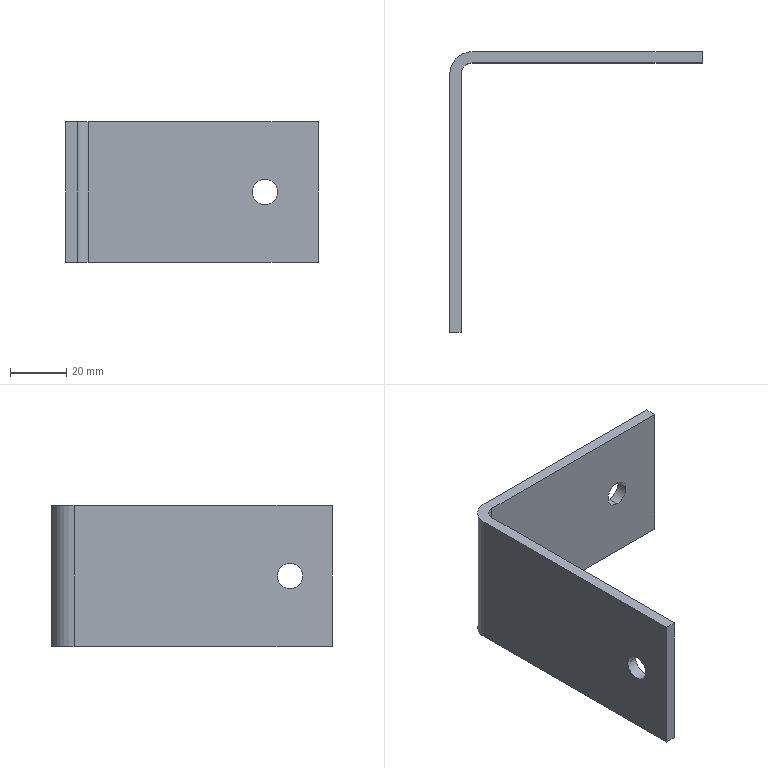Part | NX | features solid 2 | 1 solid | 14 faces | box 90 x 100 x 50 mm | volume 36176 mm3 | plane 8 | cylinder 6 | commonest cylinder face diameters 9 x4 8 x1 16 x1
STEP:
#1=CARTESIAN_POINT('',(696.5,-155.5,117.));
#2=VERTEX_POINT('',#1);
#3=CARTESIAN_POINT('',(692.5,-155.5,117.));
#4=VERTEX_POINT('',#3);
#5=CARTESIAN_POINT('',(836.027,-155.5,117.));
#6=DIRECTION('',(-1.,0.,0.));
#7=VECTOR('',#6,1000.);
#8=LINE('',#5,#7);
#9=EDGE_CURVE('',#2,#4,#8,.T.);
#10=ORIENTED_EDGE('',*,*,#9,.F.);
#11=CARTESIAN_POINT('',(696.5,-164.5,117.));
#12=VERTEX_POINT('',#11);
#13=CARTESIAN_POINT('',(696.5,-160.,117.));
#14=DIRECTION('',(-1.,0.,0.));
#15=DIRECTION('',(0.,-1.,0.));
#16=AXIS2_PLACEMENT_3D('',#13,#14,#15);
#17=CIRCLE('',#16,4.5);
#18=EDGE_CURVE('',#12,#2,#17,.T.);
#19=ORIENTED_EDGE('',*,*,#18,.F.);
#20=CARTESIAN_POINT('',(692.5,-164.5,117.));
#21=VERTEX_POINT('',#20);
#22=CARTESIAN_POINT('',(836.027,-164.5,117.));
#23=DIRECTION('',(-1.,0.,0.));
#24=VECTOR('',#23,1000.);
#25=LINE('',#22,#24);
#26=EDGE_CURVE('',#21,#12,#25,.F.);
#27=ORIENTED_EDGE('',*,*,#26,.F.);
#28=CARTESIAN_POINT('',(692.5,-160.,117.));
#29=DIRECTION('',(-1.,0.,0.));
#30=DIRECTION('',(0.,1.,0.));
#31=AXIS2_PLACEMENT_3D('',#28,#29,#30);
#32=CIRCLE('',#31,4.5);
#33=EDGE_CURVE('',#21,#4,#32,.T.);
#34=ORIENTED_EDGE('',*,*,#33,.T.);
#35=EDGE_LOOP('',(#10,#19,#27,#34));
#36=FACE_BOUND('',#35,.T.);
#37=CARTESIAN_POINT('',(836.027,-160.,117.));
#38=DIRECTION('',(-1.,0.,0.));
#39=DIRECTION('',(0.,-1.,0.));
#40=AXIS2_PLACEMENT_3D('',#37,#38,#39);
#41=CYLINDRICAL_SURFACE('',#40,4.5);
#42=ADVANCED_FACE('',(#36),#41,.F.);
#43=CARTESIAN_POINT('',(763.5,-79.,112.5));
#44=VERTEX_POINT('',#43);
#45=CARTESIAN_POINT('',(763.5,-75.,112.5));
#46=VERTEX_POINT('',#45);
#47=CARTESIAN_POINT('',(763.5,-218.527,112.5));
#48=DIRECTION('',(0.,1.,0.));
#49=VECTOR('',#48,1000.);
#50=LINE('',#47,#49);
#51=EDGE_CURVE('',#44,#46,#50,.T.);
#52=ORIENTED_EDGE('',*,*,#51,.F.);
#53=CARTESIAN_POINT('',(763.5,-79.,121.5));
#54=VERTEX_POINT('',#53);
#55=CARTESIAN_POINT('',(763.5,-79.,117.));
#56=DIRECTION('',(0.,-1.,0.));
#57=DIRECTION('',(0.,0.,-1.));
#58=AXIS2_PLACEMENT_3D('',#55,#56,#57);
#59=CIRCLE('',#58,4.5);
#60=EDGE_CURVE('',#44,#54,#59,.T.);
#61=ORIENTED_EDGE('',*,*,#60,.T.);
#62=CARTESIAN_POINT('',(763.5,-75.,121.5));
#63=VERTEX_POINT('',#62);
#64=CARTESIAN_POINT('',(763.5,-218.527,121.5));
#65=DIRECTION('',(0.,1.,0.));
#66=VECTOR('',#65,1000.);
#67=LINE('',#64,#66);
#68=EDGE_CURVE('',#63,#54,#67,.F.);
#69=ORIENTED_EDGE('',*,*,#68,.F.);
#70=CARTESIAN_POINT('',(763.5,-75.,117.));
#71=DIRECTION('',(0.,1.,0.));
#72=DIRECTION('',(1.,0.,0.));
#73=AXIS2_PLACEMENT_3D('',#70,#71,#72);
#74=CIRCLE('',#73,4.5);
#75=EDGE_CURVE('',#63,#46,#74,.T.);
#76=ORIENTED_EDGE('',*,*,#75,.T.);
#77=EDGE_LOOP('',(#52,#61,#69,#76));
#78=FACE_BOUND('',#77,.T.);
#79=CARTESIAN_POINT('',(763.5,-218.527,117.));
#80=DIRECTION('',(0.,1.,0.));
#81=DIRECTION('',(0.,0.,1.));
#82=AXIS2_PLACEMENT_3D('',#79,#80,#81);
#83=CYLINDRICAL_SURFACE('',#82,4.5);
#84=ADVANCED_FACE('',(#78),#83,.F.);
#85=CARTESIAN_POINT('',(700.5,-79.,92.));
#86=VERTEX_POINT('',#85);
#87=CARTESIAN_POINT('',(700.5,-79.,142.));
#88=VERTEX_POINT('',#87);
#89=CARTESIAN_POINT('',(700.5,-79.,92.));
#90=DIRECTION('',(0.,0.,1.));
#91=VECTOR('',#90,1000.);
#92=LINE('',#89,#91);
#93=EDGE_CURVE('',#86,#88,#92,.T.);
#94=ORIENTED_EDGE('',*,*,#93,.T.);
#95=CARTESIAN_POINT('',(696.5,-83.,142.));
#96=VERTEX_POINT('',#95);
#97=CARTESIAN_POINT('',(700.5,-83.,142.));
#98=DIRECTION('',(0.,0.,1.));
#99=DIRECTION('',(1.,0.,0.));
#100=AXIS2_PLACEMENT_3D('',#97,#98,#99);
#101=CIRCLE('',#100,4.);
#102=EDGE_CURVE('',#88,#96,#101,.T.);
#103=ORIENTED_EDGE('',*,*,#102,.T.);
#104=CARTESIAN_POINT('',(696.5,-83.,92.));
#105=VERTEX_POINT('',#104);
#106=CARTESIAN_POINT('',(696.5,-83.,142.));
#107=DIRECTION('',(0.,0.,-1.));
#108=VECTOR('',#107,1000.);
#109=LINE('',#106,#108);
#110=EDGE_CURVE('',#96,#105,#109,.T.);
#111=ORIENTED_EDGE('',*,*,#110,.T.);
#112=CARTESIAN_POINT('',(700.5,-83.,92.));
#113=DIRECTION('',(0.,0.,-1.));
#114=DIRECTION('',(1.,0.,0.));
#115=AXIS2_PLACEMENT_3D('',#112,#113,#114);
#116=CIRCLE('',#115,4.);
#117=EDGE_CURVE('',#105,#86,#116,.T.);
#118=ORIENTED_EDGE('',*,*,#117,.T.);
#119=EDGE_LOOP('',(#94,#103,#111,#118));
#120=FACE_BOUND('',#119,.T.);
#121=CARTESIAN_POINT('',(700.5,-83.,92.));
#122=DIRECTION('',(0.,0.,1.));
#123=DIRECTION('',(0.,-1.,0.));
#124=AXIS2_PLACEMENT_3D('',#121,#122,#123);
#125=CYLINDRICAL_SURFACE('',#124,4.);
#126=ADVANCED_FACE('',(#120),#125,.F.);
#127=CARTESIAN_POINT('',(700.5,-75.,92.));
#128=VERTEX_POINT('',#127);
#129=CARTESIAN_POINT('',(700.5,-75.,142.));
#130=VERTEX_POINT('',#129);
#131=CARTESIAN_POINT('',(700.5,-75.,92.));
#132=DIRECTION('',(0.,0.,1.));
#133=VECTOR('',#132,1000.);
#134=LINE('',#131,#133);
#135=EDGE_CURVE('',#128,#130,#134,.T.);
#136=ORIENTED_EDGE('',*,*,#135,.F.);
#137=CARTESIAN_POINT('',(692.5,-83.,92.));
#138=VERTEX_POINT('',#137);
#139=CARTESIAN_POINT('',(700.5,-83.,92.));
#140=DIRECTION('',(0.,0.,-1.));
#141=DIRECTION('',(0.,-1.,0.));
#142=AXIS2_PLACEMENT_3D('',#139,#140,#141);
#143=CIRCLE('',#142,8.);
#144=EDGE_CURVE('',#138,#128,#143,.T.);
#145=ORIENTED_EDGE('',*,*,#144,.F.);
#146=CARTESIAN_POINT('',(692.5,-83.,142.));
#147=VERTEX_POINT('',#146);
#148=CARTESIAN_POINT('',(692.5,-83.,142.));
#149=DIRECTION('',(0.,0.,-1.));
#150=VECTOR('',#149,1000.);
#151=LINE('',#148,#150);
#152=EDGE_CURVE('',#147,#138,#151,.T.);
#153=ORIENTED_EDGE('',*,*,#152,.F.);
#154=CARTESIAN_POINT('',(700.5,-83.,142.));
#155=DIRECTION('',(0.,0.,1.));
#156=DIRECTION('',(0.,-1.,0.));
#157=AXIS2_PLACEMENT_3D('',#154,#155,#156);
#158=CIRCLE('',#157,8.);
#159=EDGE_CURVE('',#130,#147,#158,.T.);
#160=ORIENTED_EDGE('',*,*,#159,.F.);
#161=EDGE_LOOP('',(#136,#145,#153,#160));
#162=FACE_BOUND('',#161,.T.);
#163=CARTESIAN_POINT('',(700.5,-83.,92.));
#164=DIRECTION('',(0.,0.,1.));
#165=DIRECTION('',(0.,-1.,0.));
#166=AXIS2_PLACEMENT_3D('',#163,#164,#165);
#167=CYLINDRICAL_SURFACE('',#166,8.);
#168=ADVANCED_FACE('',(#162),#167,.T.);
#169=CARTESIAN_POINT('',(696.5,-175.,92.));
#170=VERTEX_POINT('',#169);
#171=CARTESIAN_POINT('',(696.5,-175.,142.));
#172=VERTEX_POINT('',#171);
#173=CARTESIAN_POINT('',(696.5,-175.,92.));
#174=DIRECTION('',(0.,0.,1.));
#175=VECTOR('',#174,1000.);
#176=LINE('',#173,#175);
#177=EDGE_CURVE('',#170,#172,#176,.T.);
#178=ORIENTED_EDGE('',*,*,#177,.T.);
#179=CARTESIAN_POINT('',(692.5,-175.,142.));
#180=VERTEX_POINT('',#179);
#181=CARTESIAN_POINT('',(692.5,-175.,142.));
#182=DIRECTION('',(1.,0.,0.));
#183=VECTOR('',#182,1000.);
#184=LINE('',#181,#183);
#185=EDGE_CURVE('',#180,#172,#184,.T.);
#186=ORIENTED_EDGE('',*,*,#185,.F.);
#187=CARTESIAN_POINT('',(692.5,-175.,92.));
#188=VERTEX_POINT('',#187);
#189=CARTESIAN_POINT('',(692.5,-175.,92.));
#190=DIRECTION('',(0.,0.,1.));
#191=VECTOR('',#190,1000.);
#192=LINE('',#189,#191);
#193=EDGE_CURVE('',#188,#180,#192,.T.);
#194=ORIENTED_EDGE('',*,*,#193,.F.);
#195=CARTESIAN_POINT('',(692.5,-175.,92.));
#196=DIRECTION('',(1.,0.,0.));
#197=VECTOR('',#196,1000.);
#198=LINE('',#195,#197);
#199=EDGE_CURVE('',#188,#170,#198,.T.);
#200=ORIENTED_EDGE('',*,*,#199,.T.);
#201=EDGE_LOOP('',(#178,#186,#194,#200));
#202=FACE_BOUND('',#201,.T.);
#203=CARTESIAN_POINT('',(692.5,-175.,92.));
#204=DIRECTION('',(0.,1.,0.));
#205=DIRECTION('',(1.,0.,0.));
#206=AXIS2_PLACEMENT_3D('',#203,#204,#205);
#207=PLANE('',#206);
#208=ADVANCED_FACE('',(#202),#207,.F.);
#209=ORIENTED_EDGE('',*,*,#18,.T.);
#210=CARTESIAN_POINT('',(696.5,-160.,117.));
#211=DIRECTION('',(-1.,0.,0.));
#212=DIRECTION('',(0.,-1.,0.));
#213=AXIS2_PLACEMENT_3D('',#210,#211,#212);
#214=CIRCLE('',#213,4.5);
#215=EDGE_CURVE('',#2,#12,#214,.T.);
#216=ORIENTED_EDGE('',*,*,#215,.T.);
#217=EDGE_LOOP('',(#209,#216));
#218=FACE_BOUND('',#217,.T.);
#219=ORIENTED_EDGE('',*,*,#110,.F.);
#220=CARTESIAN_POINT('',(696.5,-78.445,142.));
#221=DIRECTION('',(0.,1.,0.));
#222=VECTOR('',#221,1000.);
#223=LINE('',#220,#222);
#224=EDGE_CURVE('',#172,#96,#223,.T.);
#225=ORIENTED_EDGE('',*,*,#224,.F.);
#226=ORIENTED_EDGE('',*,*,#177,.F.);
#227=CARTESIAN_POINT('',(696.5,-78.445,92.));
#228=DIRECTION('',(0.,-1.,0.));
#229=VECTOR('',#228,1000.);
#230=LINE('',#227,#229);
#231=EDGE_CURVE('',#105,#170,#230,.T.);
#232=ORIENTED_EDGE('',*,*,#231,.F.);
#233=EDGE_LOOP('',(#219,#225,#226,#232));
#234=FACE_BOUND('',#233,.T.);
#235=CARTESIAN_POINT('',(696.5,-75.,117.));
#236=DIRECTION('',(-1.,0.,0.));
#237=DIRECTION('',(0.,1.,0.));
#238=AXIS2_PLACEMENT_3D('',#235,#236,#237);
#239=PLANE('',#238);
#240=ADVANCED_FACE('',(#218,#234),#239,.F.);
#241=ORIENTED_EDGE('',*,*,#33,.F.);
#242=CARTESIAN_POINT('',(692.5,-160.,117.));
#243=DIRECTION('',(-1.,0.,0.));
#244=DIRECTION('',(0.,1.,0.));
#245=AXIS2_PLACEMENT_3D('',#242,#243,#244);
#246=CIRCLE('',#245,4.5);
#247=EDGE_CURVE('',#4,#21,#246,.T.);
#248=ORIENTED_EDGE('',*,*,#247,.F.);
#249=EDGE_LOOP('',(#241,#248));
#250=FACE_BOUND('',#249,.T.);
#251=CARTESIAN_POINT('',(692.5,-78.445,142.));
#252=DIRECTION('',(0.,1.,0.));
#253=VECTOR('',#252,1000.);
#254=LINE('',#251,#253);
#255=EDGE_CURVE('',#180,#147,#254,.T.);
#256=ORIENTED_EDGE('',*,*,#255,.T.);
#257=ORIENTED_EDGE('',*,*,#152,.T.);
#258=CARTESIAN_POINT('',(692.5,-78.445,92.));
#259=DIRECTION('',(0.,-1.,0.));
#260=VECTOR('',#259,1000.);
#261=LINE('',#258,#260);
#262=EDGE_CURVE('',#138,#188,#261,.T.);
#263=ORIENTED_EDGE('',*,*,#262,.T.);
#264=ORIENTED_EDGE('',*,*,#193,.T.);
#265=EDGE_LOOP('',(#256,#257,#263,#264));
#266=FACE_BOUND('',#265,.T.);
#267=CARTESIAN_POINT('',(692.5,-75.,117.));
#268=DIRECTION('',(-1.,0.,0.));
#269=DIRECTION('',(0.,1.,0.));
#270=AXIS2_PLACEMENT_3D('',#267,#268,#269);
#271=PLANE('',#270);
#272=ADVANCED_FACE('',(#250,#266),#271,.T.);
#273=CARTESIAN_POINT('',(763.5,-79.,117.));
#274=DIRECTION('',(0.,-1.,0.));
#275=DIRECTION('',(0.,0.,-1.));
#276=AXIS2_PLACEMENT_3D('',#273,#274,#275);
#277=CIRCLE('',#276,4.5);
#278=EDGE_CURVE('',#54,#44,#277,.T.);
#279=ORIENTED_EDGE('',*,*,#278,.F.);
#280=ORIENTED_EDGE('',*,*,#60,.F.);
#281=EDGE_LOOP('',(#279,#280));
#282=FACE_BOUND('',#281,.T.);
#283=ORIENTED_EDGE('',*,*,#93,.F.);
#284=CARTESIAN_POINT('',(782.5,-79.,92.));
#285=VERTEX_POINT('',#284);
#286=CARTESIAN_POINT('',(692.5,-79.,92.));
#287=DIRECTION('',(1.,0.,0.));
#288=VECTOR('',#287,1000.);
#289=LINE('',#286,#288);
#290=EDGE_CURVE('',#86,#285,#289,.T.);
#291=ORIENTED_EDGE('',*,*,#290,.T.);
#292=CARTESIAN_POINT('',(782.5,-79.,142.));
#293=VERTEX_POINT('',#292);
#294=CARTESIAN_POINT('',(782.5,-79.,92.));
#295=DIRECTION('',(0.,0.,1.));
#296=VECTOR('',#295,1000.);
#297=LINE('',#294,#296);
#298=EDGE_CURVE('',#285,#293,#297,.T.);
#299=ORIENTED_EDGE('',*,*,#298,.T.);
#300=CARTESIAN_POINT('',(782.5,-79.,142.));
#301=DIRECTION('',(-1.,0.,0.));
#302=VECTOR('',#301,1000.);
#303=LINE('',#300,#302);
#304=EDGE_CURVE('',#293,#88,#303,.T.);
#305=ORIENTED_EDGE('',*,*,#304,.T.);
#306=EDGE_LOOP('',(#283,#291,#299,#305));
#307=FACE_BOUND('',#306,.T.);
#308=CARTESIAN_POINT('',(737.5,-79.,117.));
#309=DIRECTION('',(0.,-1.,0.));
#310=DIRECTION('',(0.,0.,-1.));
#311=AXIS2_PLACEMENT_3D('',#308,#309,#310);
#312=PLANE('',#311);
#313=ADVANCED_FACE('',(#282,#307),#312,.T.);
#314=CARTESIAN_POINT('',(782.5,-75.,92.));
#315=VERTEX_POINT('',#314);
#316=CARTESIAN_POINT('',(782.5,-75.,142.));
#317=VERTEX_POINT('',#316);
#318=CARTESIAN_POINT('',(782.5,-75.,92.));
#319=DIRECTION('',(0.,0.,1.));
#320=VECTOR('',#319,1000.);
#321=LINE('',#318,#320);
#322=EDGE_CURVE('',#315,#317,#321,.T.);
#323=ORIENTED_EDGE('',*,*,#322,.T.);
#324=CARTESIAN_POINT('',(782.5,-79.,142.));
#325=DIRECTION('',(0.,1.,0.));
#326=VECTOR('',#325,1000.);
#327=LINE('',#324,#326);
#328=EDGE_CURVE('',#293,#317,#327,.T.);
#329=ORIENTED_EDGE('',*,*,#328,.F.);
#330=ORIENTED_EDGE('',*,*,#298,.F.);
#331=CARTESIAN_POINT('',(782.5,-79.,92.));
#332=DIRECTION('',(0.,1.,0.));
#333=VECTOR('',#332,1000.);
#334=LINE('',#331,#333);
#335=EDGE_CURVE('',#285,#315,#334,.T.);
#336=ORIENTED_EDGE('',*,*,#335,.T.);
#337=EDGE_LOOP('',(#323,#329,#330,#336));
#338=FACE_BOUND('',#337,.T.);
#339=CARTESIAN_POINT('',(782.5,-79.,92.));
#340=DIRECTION('',(-1.,0.,0.));
#341=DIRECTION('',(0.,0.,1.));
#342=AXIS2_PLACEMENT_3D('',#339,#340,#341);
#343=PLANE('',#342);
#344=ADVANCED_FACE('',(#338),#343,.F.);
#345=ORIENTED_EDGE('',*,*,#75,.F.);
#346=CARTESIAN_POINT('',(763.5,-75.,117.));
#347=DIRECTION('',(0.,1.,0.));
#348=DIRECTION('',(1.,0.,0.));
#349=AXIS2_PLACEMENT_3D('',#346,#347,#348);
#350=CIRCLE('',#349,4.5);
#351=EDGE_CURVE('',#46,#63,#350,.T.);
#352=ORIENTED_EDGE('',*,*,#351,.F.);
#353=EDGE_LOOP('',(#345,#352));
#354=FACE_BOUND('',#353,.T.);
#355=CARTESIAN_POINT('',(692.5,-75.,92.));
#356=DIRECTION('',(1.,0.,0.));
#357=VECTOR('',#356,1000.);
#358=LINE('',#355,#357);
#359=EDGE_CURVE('',#128,#315,#358,.T.);
#360=ORIENTED_EDGE('',*,*,#359,.F.);
#361=ORIENTED_EDGE('',*,*,#135,.T.);
#362=CARTESIAN_POINT('',(782.5,-75.,142.));
#363=DIRECTION('',(-1.,0.,0.));
#364=VECTOR('',#363,1000.);
#365=LINE('',#362,#364);
#366=EDGE_CURVE('',#317,#130,#365,.T.);
#367=ORIENTED_EDGE('',*,*,#366,.F.);
#368=ORIENTED_EDGE('',*,*,#322,.F.);
#369=EDGE_LOOP('',(#360,#361,#367,#368));
#370=FACE_BOUND('',#369,.T.);
#371=CARTESIAN_POINT('',(737.5,-75.,117.));
#372=DIRECTION('',(0.,-1.,0.));
#373=DIRECTION('',(0.,0.,-1.));
#374=AXIS2_PLACEMENT_3D('',#371,#372,#373);
#375=PLANE('',#374);
#376=ADVANCED_FACE('',(#354,#370),#375,.F.);
#377=ORIENTED_EDGE('',*,*,#366,.T.);
#378=ORIENTED_EDGE('',*,*,#159,.T.);
#379=ORIENTED_EDGE('',*,*,#255,.F.);
#380=ORIENTED_EDGE('',*,*,#185,.T.);
#381=ORIENTED_EDGE('',*,*,#224,.T.);
#382=ORIENTED_EDGE('',*,*,#102,.F.);
#383=ORIENTED_EDGE('',*,*,#304,.F.);
#384=ORIENTED_EDGE('',*,*,#328,.T.);
#385=EDGE_LOOP('',(#377,#378,#379,#380,#381,#382,#383,#384));
#386=FACE_BOUND('',#385,.T.);
#387=CARTESIAN_POINT('',(782.5,-79.,142.));
#388=DIRECTION('',(0.,0.,-1.));
#389=DIRECTION('',(0.,-1.,0.));
#390=AXIS2_PLACEMENT_3D('',#387,#388,#389);
#391=PLANE('',#390);
#392=ADVANCED_FACE('',(#386),#391,.F.);
#393=ORIENTED_EDGE('',*,*,#290,.F.);
#394=ORIENTED_EDGE('',*,*,#117,.F.);
#395=ORIENTED_EDGE('',*,*,#231,.T.);
#396=ORIENTED_EDGE('',*,*,#199,.F.);
#397=ORIENTED_EDGE('',*,*,#262,.F.);
#398=ORIENTED_EDGE('',*,*,#144,.T.);
#399=ORIENTED_EDGE('',*,*,#359,.T.);
#400=ORIENTED_EDGE('',*,*,#335,.F.);
#401=EDGE_LOOP('',(#393,#394,#395,#396,#397,#398,#399,#400));
#402=FACE_BOUND('',#401,.T.);
#403=CARTESIAN_POINT('',(692.5,-79.,92.));
#404=DIRECTION('',(0.,0.,1.));
#405=DIRECTION('',(1.,0.,0.));
#406=AXIS2_PLACEMENT_3D('',#403,#404,#405);
#407=PLANE('',#406);
#408=ADVANCED_FACE('',(#402),#407,.F.);
#409=ORIENTED_EDGE('',*,*,#278,.T.);
#410=ORIENTED_EDGE('',*,*,#51,.T.);
#411=ORIENTED_EDGE('',*,*,#351,.T.);
#412=ORIENTED_EDGE('',*,*,#68,.T.);
#413=EDGE_LOOP('',(#409,#410,#411,#412));
#414=FACE_BOUND('',#413,.T.);
#415=CARTESIAN_POINT('',(763.5,-218.527,117.));
#416=DIRECTION('',(0.,1.,0.));
#417=DIRECTION('',(0.,0.,1.));
#418=AXIS2_PLACEMENT_3D('',#415,#416,#417);
#419=CYLINDRICAL_SURFACE('',#418,4.5);
#420=ADVANCED_FACE('',(#414),#419,.F.);
#421=ORIENTED_EDGE('',*,*,#215,.F.);
#422=ORIENTED_EDGE('',*,*,#9,.T.);
#423=ORIENTED_EDGE('',*,*,#247,.T.);
#424=ORIENTED_EDGE('',*,*,#26,.T.);
#425=EDGE_LOOP('',(#421,#422,#423,#424));
#426=FACE_BOUND('',#425,.T.);
#427=CARTESIAN_POINT('',(836.027,-160.,117.));
#428=DIRECTION('',(-1.,0.,0.));
#429=DIRECTION('',(0.,-1.,0.));
#430=AXIS2_PLACEMENT_3D('',#427,#428,#429);
#431=CYLINDRICAL_SURFACE('',#430,4.5);
#432=ADVANCED_FACE('',(#426),#431,.F.);
#433=CLOSED_SHELL('',(#42,#84,#126,#168,#208,#240,#272,#313,#344,#376,#392,#408,#420,#432));
#434=MANIFOLD_SOLID_BREP('',#433);
#435=(LENGTH_UNIT()NAMED_UNIT(*)SI_UNIT(.MILLI.,.METRE.));
#436=UNCERTAINTY_MEASURE_WITH_UNIT(LENGTH_MEASURE(0.00001),#435,'','');
#437=(NAMED_UNIT(*)PLANE_ANGLE_UNIT()SI_UNIT($,.RADIAN.));
#438=(NAMED_UNIT(*)SI_UNIT($,.STERADIAN.)SOLID_ANGLE_UNIT());
#439=(GEOMETRIC_REPRESENTATION_CONTEXT(3)GLOBAL_UNCERTAINTY_ASSIGNED_CONTEXT((#436))GLOBAL_UNIT_ASSIGNED_CONTEXT((#435,#437,#438))REPRESENTATION_CONTEXT('',''));
#440=ADVANCED_BREP_SHAPE_REPRESENTATION('',(#434),#439);